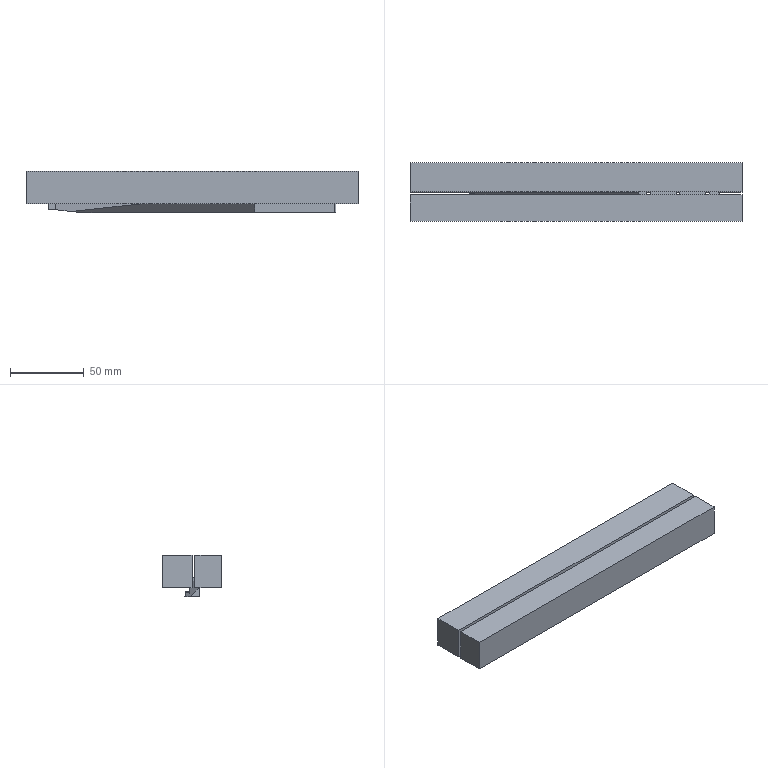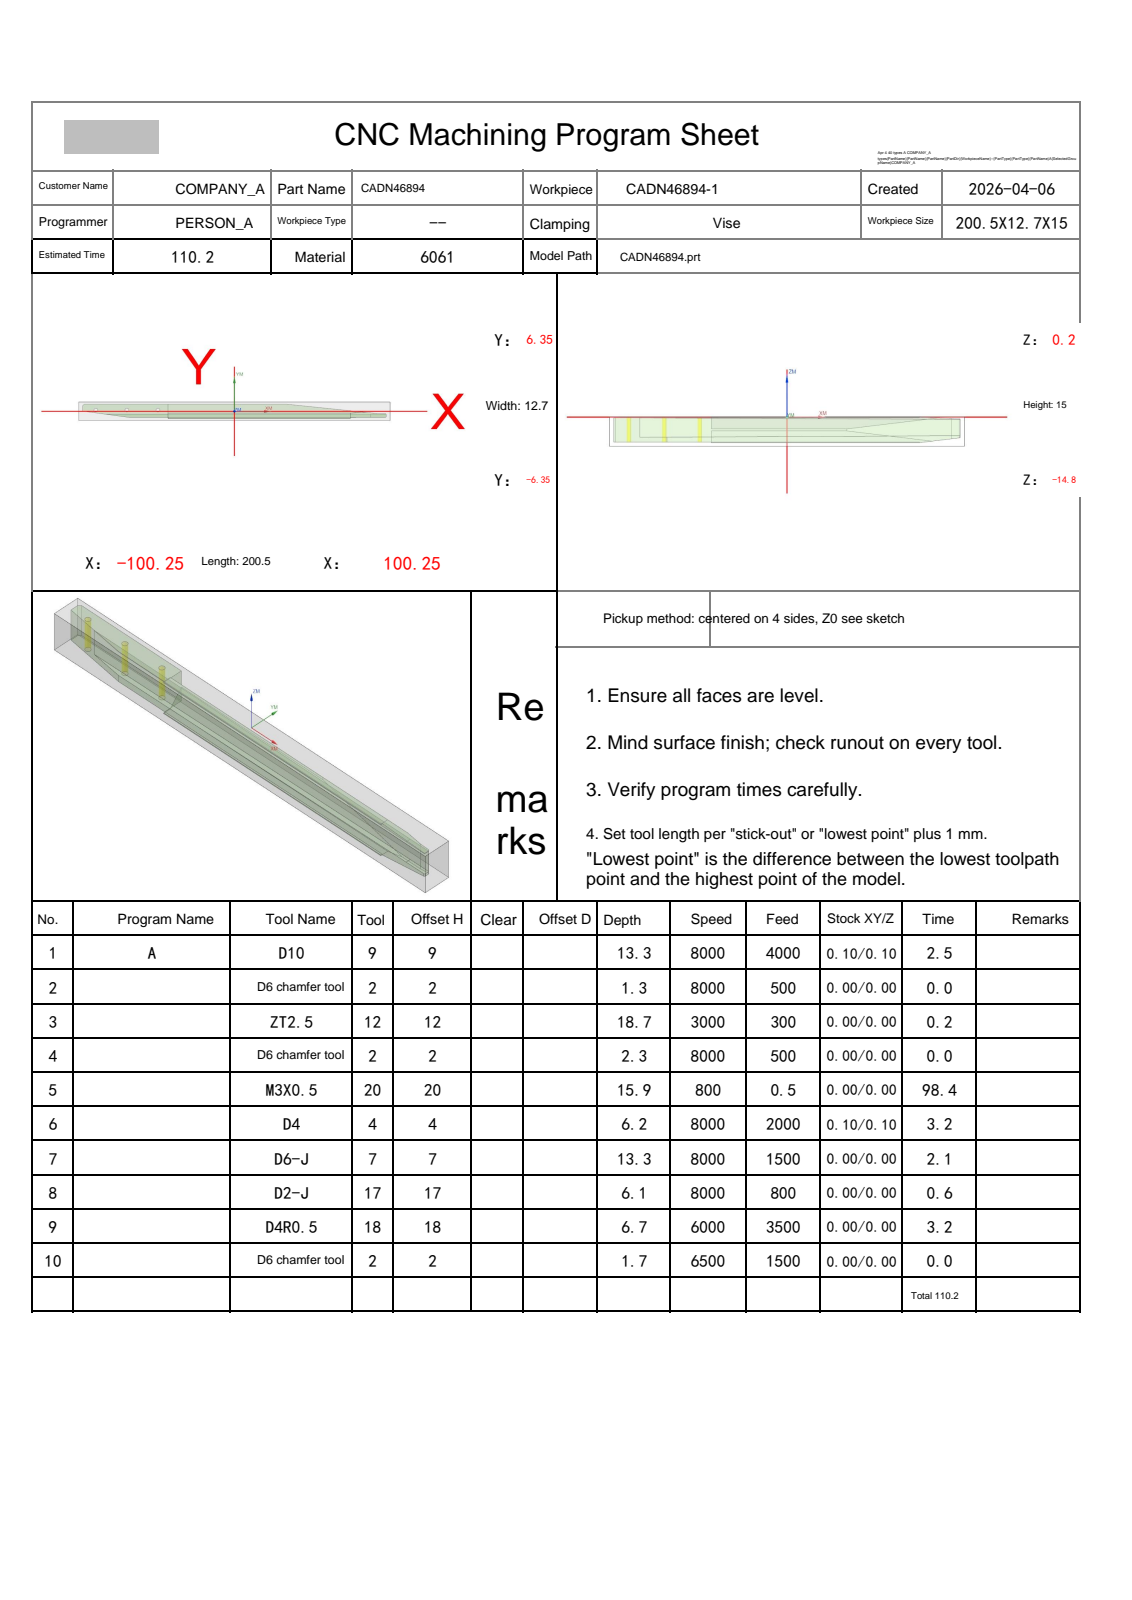NC program | NX | posted by the shop | part box 225.5 x 39.7 x 28 mm
Lines 1 to 2327 of 2996, first 1800 of 2325 lines:
%
O0001
(Machine time: 10.65 MIN)
(===Total Tool:5===)
(T4=D4      D=4.   R=0.   D-  H04 Z=-6.   )
(T7=D6-J    D=6.   R=0.   D7  H07 Z=-0.3  )
(T17=D2-J   D=2.   R=0.   D-  H17 Z=-5.9  )
(T2=D6 chamfer tool   D=6.   R=0.   D-  H02 Z=-1.5  )
(T18=D4R0.5 D=4.   R=0.5  D-  H18 Z=-6.43 )
G80 G90 G17 G49 G40
G91 G28 Z0
M01
N1 T04 M06
(D4  D=4. R=0. H=04 ce=0.20 di=0.10)
G00 G90 G54 X-209.5 Y-.74 M03 S4500
G43 H04 Z50.
M08
Z3.729
G01 Z1.729 F3000.
X-197.5
X1.601
G02 X2. Y-1.139 I-.001 J-.4
G01 Y-3.08
G02 X1.6 Y-3.48 I-.4 J0.0
G01 X-197.101
G03 X-197.5 Y-3.879 I.001 J-.4
G01 Y-5.86
G03 X-197.14 Y-6.22 I.36 J0.0
G01 X1.601
G02 X2. Y-6.619 I-.001 J-.4
G01 Y-8.56
G02 X1.6 Y-8.96 I-.4 J0.0
G01 X-197.5
X-209.5
Z3.729
G00 Z5.
Y-.74
Z3.457
G01 Z1.457
X-197.5
X1.601
G02 X2. Y-1.139 I-.001 J-.4
G01 Y-3.08
G02 X1.6 Y-3.48 I-.4 J0.0
G01 X-197.101
G03 X-197.5 Y-3.879 I.001 J-.4
G01 Y-5.86
G03 X-197.14 Y-6.22 I.36 J0.0
G01 X1.601
G02 X2. Y-6.619 I-.001 J-.4
G01 Y-8.56
G02 X1.6 Y-8.96 I-.4 J0.0
G01 X-197.5
X-209.5
Z3.457
G00 Z4.729
Y-.74
Z3.186
G01 Z1.186
X-197.5
X1.601
G02 X2. Y-1.139 I-.001 J-.4
G01 Y-3.08
G02 X1.6 Y-3.48 I-.4 J0.0
G01 X-197.101
G03 X-197.5 Y-3.879 I.001 J-.4
G01 Y-5.86
G03 X-197.14 Y-6.22 I.36 J0.0
G01 X1.601
G02 X2. Y-6.619 I-.001 J-.4
G01 Y-8.56
G02 X1.6 Y-8.96 I-.4 J0.0
G01 X-197.5
X-209.5
Z3.186
G00 Z4.457
Y-.74
Z2.914
G01 Z.914
X-197.5
X1.601
G02 X2. Y-1.139 I-.001 J-.4
G01 Y-3.08
G02 X1.6 Y-3.48 I-.4 J0.0
G01 X-197.101
G03 X-197.5 Y-3.879 I.001 J-.4
G01 Y-5.86
G03 X-197.14 Y-6.22 I.36 J0.0
G01 X1.601
G02 X2. Y-6.619 I-.001 J-.4
G01 Y-8.56
G02 X1.6 Y-8.96 I-.4 J0.0
G01 X-197.5
X-209.5
Z2.914
G00 Z4.186
Y-.74
Z2.643
G01 Z.643
X-197.5
X1.601
G02 X2. Y-1.139 I-.001 J-.4
G01 Y-3.08
G02 X1.6 Y-3.48 I-.4 J0.0
G01 X-197.101
G03 X-197.5 Y-3.879 I.001 J-.4
G01 Y-5.86
G03 X-197.14 Y-6.22 I.36 J0.0
G01 X1.601
G02 X2. Y-6.619 I-.001 J-.4
G01 Y-8.56
G02 X1.6 Y-8.96 I-.4 J0.0
G01 X-197.5
X-209.5
Z2.643
G00 Z3.914
Y-.74
Z2.371
G01 Z.371
X-197.5
X1.601
G02 X2. Y-1.139 I-.001 J-.4
G01 Y-3.08
G02 X1.6 Y-3.48 I-.4 J0.0
G01 X-197.101
G03 X-197.5 Y-3.879 I.001 J-.4
G01 Y-5.86
G03 X-197.14 Y-6.22 I.36 J0.0
G01 X1.601
G02 X2. Y-6.619 I-.001 J-.4
G01 Y-8.56
G02 X1.6 Y-8.96 I-.4 J0.0
G01 X-197.5
X-209.5
Z2.371
G00 Z3.643
Y-.74
Z2.1
G01 Z.1
X-197.5
X1.601
G02 X2. Y-1.139 I-.001 J-.4
G01 Y-3.08
G02 X1.6 Y-3.48 I-.4 J0.0
G01 X-197.101
G03 X-197.5 Y-3.879 I.001 J-.4
G01 Y-5.86
G03 X-197.14 Y-6.22 I.36 J0.0
G01 X1.601
G02 X2. Y-6.619 I-.001 J-.4
G01 Y-8.56
G02 X1.6 Y-8.96 I-.4 J0.0
G01 X-197.5
X-209.5
Z2.1
G00 Z50.
G00 G90 X-196.166 Y-14.577 M03 S8000
Z11.8
Z1.3
G01 Z-.2 F4000.
X-196.501 Y-10.471
G02 X-196.68 Y-6.08 I53.821 J4.391
G01 Y-3.536
G02 X-196.337 Y-3.14 I.4 J0.0
G01 X-194.045 Y-2.811
X-194. Y-2.808
G02 X-193.68 Y-3.128 I0.0 J-.32
G01 Y-6.08
G03 X-193.412 Y-11.301 I51. J0.0
X-193.014 Y-11.66 I.398 J.041
G01 X-190.713
G03 X-190.393 Y-11.34 I0.0 J.32
G01 X-190.395 Y-11.305
G02 X-190.68 Y-6.08 I47.715 J5.225
G01 Y-2.676
G02 X-190.337 Y-2.28 I.4 J0.0
G01 X-188.045 Y-1.951
X-188. Y-1.948
G02 X-187.68 Y-2.268 I0.0 J-.32
G01 Y-6.08
G03 X-187.375 Y-11.307 I45. J0.0
X-186.978 Y-11.66 I.397 J.047
G01 X-184.672
G03 X-184.352 Y-11.34 I0.0 J.32
G01 X-184.354 Y-11.3
G02 X-184.68 Y-6.08 I41.674 J5.22
G01 Y-1.816
G02 X-184.337 Y-1.42 I.4 J0.0
G01 X-182.045 Y-1.091
X-182. Y-1.088
G02 X-181.68 Y-1.408 I0.0 J-.32
G01 Y-6.08
G03 X-181.327 Y-11.314 I39. J0.0
X-180.931 Y-11.66 I.396 J.054
G01 X-178.617
G03 X-178.297 Y-11.34 I0.0 J.32
G01 X-178.3 Y-11.294
G02 X-178.68 Y-6.08 I35.62 J5.214
G01 Y-.956
G02 X-178.337 Y-.56 I.4 J0.0
G01 X-176.045 Y-.231
X-176. Y-.228
G02 X-175.68 Y-.548 I0.0 J-.32
G01 Y-6.08
G03 X-175.261 Y-11.324 I33. J0.0
X-174.866 Y-11.66 I.395 J.064
G01 X-172.54
G03 X-172.22 Y-11.34 I0.0 J.32
G01 X-172.225 Y-11.285
G02 X-172.68 Y-6.08 I29.545 J5.205
G01 Y-.096
G02 X-172.337 Y.3 I.4 J0.0
G01 X-170.045 Y.629
X-170. Y.632
G02 X-169.68 Y.312 I0.0 J-.32
G01 Y-6.08
G03 X-169.163 Y-11.338 I27. J0.0
X-168.771 Y-11.66 I.392 J.078
G01 X-166.374
G03 X-166.094 Y-11.38 I0.0 J.28
G01 X-166.101 Y-11.319
G02 X-166.68 Y-6.08 I23.421 J5.239
G01 Y.764
G02 X-166.337 Y1.16 I.4 J0.0
G01 X-165.668 Y1.256
X-165.611 Y1.26
X-164.08
G02 X-163.68 Y.86 I0.0 J-.4
G01 Y-6.08
G03 X-163.005 Y-11.361 I21. J0.0
X-162.618 Y-11.66 I.387 J.101
G01 X-160.175
G03 X-159.895 Y-11.38 I0.0 J.28
G01 X-159.907 Y-11.299
G02 X-160.68 Y-6.08 I17.227 J5.219
G01 Y.86
G02 X-160.28 Y1.26 I.4 J0.0
G01 X-158.08
G02 X-157.68 Y.86 I0.0 J-.4
G01 Y-6.08
G03 X-156.704 Y-11.402 I15. J0.0
X-156.33 Y-11.66 I.374 J.142
G01 X-153.694
G03 X-153.454 Y-11.42 I0.0 J.24
G01 X-153.478 Y-11.315
G02 X-154.68 Y-6.08 I10.798 J5.235
G01 Y.86
G02 X-154.28 Y1.26 I.4 J0.0
G01 X-152.08
G02 X-151.68 Y.86 I0.0 J-.4
G01 Y-6.08
G03 X-149.864 Y-11.501 I9. J0.0
X-149.545 Y-11.66 I.319 J.241
G01 X-145.272
X-145.192 Y-11.58
X-145.237 Y-11.508
G02 X-148.68 Y-6.08 I2.557 J5.428
G01 Y.86
G02 X-148.28 Y1.26 I.4 J0.0
G01 X-146.08
G02 X-145.68 Y.86 I0.0 J-.4
G01 Y-6.08
G03 X-142.68 Y-9.08 I3. J0.0
G01 X-138.882
G03 X-138.487 Y-8.742 I0.0 J.4
G01 X-138.145 Y-6.542
X-138.14 Y-6.48
G03 X-138.54 Y-6.08 I-.4 J0.0
G01 X-142.68
Y1.26
Y5.18
Z1.3
G00 Z11.8
G00 G90 X-88.285 Y-14.646 M03 S8000
Z11.8
Z.9
G01 Z-.3 F2000.
Y-14.2
G03 X-91.085 Y-11.4 I-2.8 J0.0
G01 X-138.458
G02 X-138.92 Y-11.836 I-2.056 J1.714
G01 X-140.071
X-140.147 Y-11.849
X-140.15 Y-11.771
G03 X-138.398 Y-9.686 I-.365 J2.085
G01 X-138.4 Y-9.589
X-138.321 Y-9.588
X-138.324 Y-6.236
X-138.333 Y-6.141
X-19.589
X-19.473 Y-6.145
G03 X-17.315 Y-4.099 I0.0 J2.162
G01 Y-.78
Y-.62
X.975
X1.83 Y-.628
X1.896 Y-.608
X1.903 Y-.677
X2.083 Y-1.121
X2.091 Y-1.226
Y-2.343
X2.08 Y-2.904
X2.066 Y-3.114
X2.084 Y-3.176
X2.019 Y-3.181
X1.867 Y-3.25
X1.561 Y-3.374
X1.531 Y-3.38
X-2.97 Y-3.379
X-12.736 Y-4.438
X-12.779 Y-4.44
G02 X-12.98 Y-4.386 I0.0 J.4
G01 X-14.792 Y-3.332
G03 X-14.993 Y-3.278 I-.201 J-.346
G01 X-15.105 Y-3.294
X-15.195 Y-3.307
G02 X-15.515 Y-2.988 I0.0 J.32
G01 Y-2.779
G02 X-15.156 Y-2.42 I.36 J-.002
G01 X-12.308
X-12.228 Y-2.5
X-12.299 Y-2.58
X-13.804 Y-2.743
G03 X-14.161 Y-3.141 I.043 J-.398
G01 X-14.159 Y-3.178
X-13.959 Y-5.302
X-13.957 Y-5.339
G02 X-14.064 Y-5.611 I-.4 J0.0
G01 X-14.205 Y-5.764
X-14.779 Y-6.274
X-15.027 Y-6.432
X-15.371 Y-6.524
X-15.942 Y-6.636
X-59.845 Y-11.4
X-93.085
G02 X-93.463 Y-11.129 I0.0 J.4
G01 X-93.892 Y-9.871
G03 X-94.27 Y-9.6 I-.378 J-.129
G01 X-136.123
G02 X-136.522 Y-9.202 I.002 J.4
G01 Y-8.34
G02 X-136.124 Y-7.941 I.4 J-.001
G01 X-46.135
X-46.056 Y-8.021
X-46.127 Y-8.101
X-59.962 Y-9.6
X-93.085
X-93.585
G03 X-96.385 Y-12.4 I0.0 J-2.8
G01 Y-14.645
Z.9
G00 Z3.
G01 X-89.675 Y-14.646 F6000.
G00 Z.6
G01 Z-.6 F2000.
Y-14.2
G03 X-92.475 Y-11.4 I-2.8 J0.0
G01 X-138.454
G02 X-138.915 Y-11.836 I-2.046 J1.7
G01 X-140.071
X-140.147 Y-11.849
X-140.15 Y-11.771
X-140.013 Y-11.743
G03 X-138.435 Y-10.083 I-.487 J2.043
X-138.398 Y-9.686 I-2.079 J.397
G01 X-138.4 Y-9.598
X-138.321 Y-9.597
X-138.322 Y-9.203
X-138.323 Y-7.001
X-138.324 Y-6.441
X-16.829
X-16.713 Y-6.445
G03 X-14.555 Y-4.399 I0.0 J2.162
G01 Y-.78
Y-.701
X-14.554 Y-.7
X-14.555 Y-.674
Y-.673
Y-.62
X.975
X1.83 Y-.628
X1.896 Y-.608
X1.903 Y-.677
X2.083 Y-1.121
X2.091 Y-1.226
Y-2.343
X2.08 Y-2.904
X2.066 Y-3.114
X2.084 Y-3.176
X2.019 Y-3.181
X1.867 Y-3.25
X1.561 Y-3.374
X1.531 Y-3.38
X-2.97 Y-3.379
X-11.332 Y-4.286
X-11.375 Y-4.288
G02 X-11.712 Y-4.104 I0.0 J.4
G01 X-12.577 Y-2.76
G03 X-12.722 Y-2.604 I-.499 J-.321
G01 X-12.781 Y-2.595
X-12.755 Y-2.541
Y-2.5
X-12.759 Y-2.415
X-12.675 Y-2.42
X-12.307
X-12.22 Y-2.419
X-12.189 Y-2.509
X-12.258 Y-2.563
X-12.35 Y-2.672
X-13.267 Y-4.325
G02 X-13.574 Y-4.528 I-.35 J.194
G01 X-13.761 Y-4.549
X-13.879 Y-5.147
X-13.96 Y-5.484
X-13.979 Y-5.52
X-14.205 Y-5.764
X-14.779 Y-6.274
X-15.027 Y-6.432
X-15.052 Y-6.439
X-15.371 Y-6.524
X-15.942 Y-6.636
X-19.31 Y-7.001
X-59.845 Y-11.4
X-94.475
G02 X-94.854 Y-11.129 I0.0 J.4
G01 X-95.283 Y-9.871
G03 X-95.661 Y-9.6 I-.378 J-.129
G01 X-136.124
G02 X-136.522 Y-9.202 I.002 J.4
G01 Y-8.64
G02 X-136.124 Y-8.241 I.4 J-.002
G01 X-48.9
X-48.821 Y-8.321
X-48.891 Y-8.401
X-59.962 Y-9.6
X-94.475
X-94.975
G03 X-97.775 Y-12.4 I0.0 J-2.8
G01 Y-14.644
Z.6
G00 Z2.7
G01 X-91.066 Y-14.646 F6000.
G00 Z.3
G01 Z-.9 F2000.
Y-14.2
G03 X-93.866 Y-11.4 I-2.8 J0.0
G01 X-138.454
G02 X-138.915 Y-11.836 I-2.046 J1.7
G01 X-140.071
X-140.147 Y-11.849
X-140.15 Y-11.771
X-140.013 Y-11.743
G03 X-138.435 Y-10.083 I-.487 J2.043
X-138.398 Y-9.686 I-2.079 J.397
G01 X-138.399 Y-9.607
X-138.321 Y-9.606
X-138.322 Y-9.204
X-138.323 Y-6.741
X-17.636
X-16.758 Y-6.688
X-15.524 Y-6.554
X-15.942 Y-6.636
X-59.845 Y-11.4
X-95.866
G02 X-96.244 Y-11.129 I0.0 J.4
G01 X-96.673 Y-9.871
G03 X-97.051 Y-9.6 I-.378 J-.129
G01 X-136.124
G02 X-136.522 Y-9.202 I.002 J.4
G01 Y-8.94
G02 X-136.124 Y-8.541 I.4 J-.002
G01 X-51.665
X-51.585 Y-8.621
X-51.656 Y-8.701
X-59.962 Y-9.6
X-95.866
X-96.366
G03 X-99.166 Y-12.4 I0.0 J-2.8
G01 Y-14.644
Z.3
G00 Z2.4
G01 X-92.476 Y-14.645 F6000.
G00 Z0.0
G01 Z-1.2 F2000.
Y-14.2
G03 X-95.276 Y-11.4 I-2.8 J0.0
G01 X-138.454
G02 X-138.915 Y-11.836 I-2.046 J1.7
G01 X-140.071
X-140.147 Y-11.849
X-140.15 Y-11.771
X-140.013 Y-11.743
G03 X-138.435 Y-10.083 I-.487 J2.043
X-138.398 Y-9.686 I-2.079 J.397
G01 X-138.399 Y-9.617
X-138.321 Y-9.616
X-138.322 Y-9.244
X-138.323 Y-7.041
X-20.402
X-19.336 Y-6.967
X-15.524 Y-6.554
X-15.533 Y-6.556
X-15.942 Y-6.636
X-24.839 Y-7.601
X-59.845 Y-11.4
X-97.276
G02 X-97.654 Y-11.129 I0.0 J.4
G01 X-98.084 Y-9.871
G03 X-98.462 Y-9.6 I-.378 J-.129
G01 X-136.164
G02 X-136.524 Y-9.238 I.002 J.362
G01 X-136.522 Y-9.2
G02 X-136.164 Y-8.841 I.36 J-.002
G01 X-54.429
X-54.35 Y-8.921
X-54.42 Y-9.001
X-59.959 Y-9.6
X-97.276
X-97.776
G03 X-100.576 Y-12.4 I0.0 J-2.8
G01 Y-14.644
Z0.0
G00 Z2.1
G01 X-93.946 Y-14.645 F6000.
G00 Z-.3
G01 Z-1.5 F2000.
Y-14.2
G03 X-96.746 Y-11.4 I-2.8 J0.0
G01 X-138.454
G02 X-138.915 Y-11.836 I-2.046 J1.7
G01 X-140.071
X-140.147 Y-11.849
X-140.15 Y-11.771
X-140.013 Y-11.743
G03 X-138.435 Y-10.083 I-.487 J2.043
X-138.398 Y-9.686 I-2.079 J.397
G01 X-138.399 Y-9.626
X-138.321 Y-9.625
X-138.322 Y-9.403
X-138.323 Y-7.341
X-23.167
X-21.593 Y-7.212
X-16.606 Y-6.671
X-15.524 Y-6.554
X-15.533 Y-6.556
X-15.942 Y-6.636
X-59.845 Y-11.4
X-98.746
G02 X-99.125 Y-11.129 I0.0 J.4
G01 X-99.554 Y-9.871
G03 X-99.932 Y-9.6 I-.378 J-.129
G01 X-136.323
G02 X-136.522 Y-9.402 I.002 J.2
G01 Y-9.34
G02 X-136.323 Y-9.141 I.2 J-.001
G01 X-57.194
X-57.115 Y-9.221
X-57.185 Y-9.301
X-59.951 Y-9.6
X-98.746
X-99.246
G03 X-102.046 Y-12.4 I0.0 J-2.8
G01 Y-14.644
Z-.3
G00 Z1.8
G01 X-74.061 Y-14.649 F6000.
G00 Z-.6
G01 Z-1.8 F2000.
Y-14.2
G03 X-76.861 Y-11.4 I-2.8 J0.0
G01 X-138.454
G02 X-138.915 Y-11.836 I-2.046 J1.7
G01 X-140.071
X-140.147 Y-11.849
X-140.15 Y-11.771
X-140.013 Y-11.743
G03 X-138.435 Y-10.083 I-.487 J2.043
X-138.398 Y-9.686 I-2.079 J.397
G01 Y-9.636
X-138.321 Y-9.634
X-138.323 Y-7.641
X-25.933
X-25.055 Y-7.588
X-16.015 Y-6.607
X-15.524 Y-6.554
X-15.533 Y-6.556
X-15.781 Y-6.604
X-15.942 Y-6.636
X-28.475 Y-7.996
X-30.369 Y-8.201
X-59.845 Y-11.4
X-76.861
X-77.361
G03 X-80.161 Y-14.2 I0.0 J-2.8
G01 Y-14.648
Z-.6
G00 Z1.5
G01 X-74.061 Y-14.649 F6000.
G00 Z-.9
G01 Z-2.1 F2000.
Y-14.2
G03 X-76.861 Y-11.4 I-2.8 J0.0
G01 X-138.454
G02 X-138.915 Y-11.836 I-2.046 J1.7
G01 X-140.071
X-140.147 Y-11.849
X-140.15 Y-11.771
X-140.013 Y-11.743
G03 X-138.435 Y-10.083 I-.487 J2.043
X-138.398 Y-9.686 I-2.079 J.397
G01 Y-9.645
X-138.321 Y-9.644
X-138.322 Y-8.81
Y-8.501
X-138.323 Y-7.941
X-28.699
X-27.821 Y-7.888
X-25.055 Y-7.588
X-22.1 Y-7.267
X-18.812 Y-6.911
X-15.524 Y-6.554
X-15.533 Y-6.556
X-15.942 Y-6.636
X-59.845 Y-11.4
X-76.861
X-77.361
G03 X-80.161 Y-14.2 I0.0 J-2.8
G01 Y-14.648
Z-.9
G00 Z1.2
G01 X-74.061 Y-14.649 F6000.
G00 Z-1.2
G01 Z-2.4 F2000.
Y-14.2
G03 X-76.861 Y-11.4 I-2.8 J0.0
G01 X-138.454
G02 X-138.915 Y-11.836 I-2.046 J1.7
G01 X-140.071
X-140.147 Y-11.849
X-140.15 Y-11.771
X-140.013 Y-11.743
G03 X-138.435 Y-10.083 I-.487 J2.043
X-138.398 Y-9.686 I-2.079 J.397
G01 Y-9.654
X-138.321 Y-9.653
X-138.322 Y-8.241
X-31.519
X-30.586 Y-8.188
X-16.998 Y-6.714
X-15.524 Y-6.554
X-15.533 Y-6.556
X-15.942 Y-6.636
X-59.845 Y-11.4
X-76.861
X-77.361
G03 X-80.161 Y-14.2 I0.0 J-2.8
G01 Y-14.648
Z-1.2
G00 Z.9
G01 X-84.266 Y-14.647 F6000.
G00 Z-1.5
G01 Z-2.7 F2000.
G03 X-87.066 Y-11.846 I-2.8 J0.0
G01 X-140.071 Y-11.836
X-140.147 Y-11.849
X-140.15 Y-11.771
X-140.013 Y-11.743
G03 X-138.435 Y-10.083 I-.487 J2.043
X-138.398 Y-9.686 I-2.079 J.397
G01 Y-9.664
X-138.32 Y-9.663
X-138.322 Y-8.541
X-34.244 Y-8.538
X-34.235 Y-8.621
X-63.905 Y-11.84
X-64.471 Y-11.851
X-87.066 Y-11.846
X-87.566
G03 X-90.366 Y-14.646 I0.0 J-2.8
G01 Z-1.5
G00 Z.6
G01 X-84.266 Y-14.647 F6000.
G00 Z-1.8
G01 Z-3. F2000.
G03 X-87.066 Y-11.846 I-2.8 J0.0
G01 X-140.071 Y-11.836
X-140.147 Y-11.849
X-140.15 Y-11.771
X-139.973 Y-11.733
G03 X-138.435 Y-10.083 I-.527 J2.033
X-138.398 Y-9.686 I-2.079 J.397
G01 Y-9.673
X-138.32 Y-9.672
X-138.321 Y-9.588
X-138.322 Y-8.841
X-37.144
X-37.008 Y-8.834
X-36.999 Y-8.921
X-63.905 Y-11.84
X-64.471 Y-11.851
X-87.066 Y-11.846
X-87.566
G03 X-90.366 Y-14.646 I0.0 J-2.8
G01 Z-1.8
G00 Z.3
G01 X-84.266 Y-14.647 F6000.
G00 Z-2.1
G01 Z-3.3 F2000.
G03 X-87.066 Y-11.846 I-2.8 J0.0
G01 X-140.071 Y-11.836
X-140.147 Y-11.849
X-140.15 Y-11.771
X-140.013 Y-11.743
G03 X-138.435 Y-10.083 I-.487 J2.043
X-138.398 Y-9.686 I-2.079 J.396
G01 Y-9.682
X-138.32 Y-9.681
X-138.321 Y-9.588
X-138.322 Y-9.141
X-39.919
X-39.773 Y-9.134
X-39.763 Y-9.221
X-63.905 Y-11.84
X-64.471 Y-11.851
X-87.066 Y-11.846
X-87.566
G03 X-90.366 Y-14.646 I0.0 J-2.8
G01 Z-2.1
G00 Z0.0
G01 X-84.266 Y-14.647 F6000.
G00 Z-2.4
G01 Z-3.6 F2000.
G03 X-87.066 Y-11.846 I-2.8 J0.0
G01 X-140.071 Y-11.836
X-140.147 Y-11.849
X-140.15 Y-11.771
X-140.013 Y-11.743
G03 X-138.435 Y-10.083 I-.487 J2.043
X-138.398 Y-9.692 I-2.079 J.396
G01 X-138.32 Y-9.691
X-138.321 Y-9.588
X-138.322 Y-9.441
X-42.537
X-42.528 Y-9.521
X-63.905 Y-11.84
X-64.471 Y-11.851
X-87.066 Y-11.846
X-87.566
G03 X-90.366 Y-14.646 I0.0 J-2.8
G01 Z-2.4
G00 Z-.3
G01 X-84.266 Y-14.647 F6000.
G00 Z-2.7
G01 Z-3.9 F2000.
G03 X-87.066 Y-11.846 I-2.8 J0.0
G01 X-140.071 Y-11.836
X-140.147 Y-11.849
X-140.15 Y-11.771
X-140.013 Y-11.743
G03 X-138.435 Y-10.083 I-.487 J2.043
X-138.398 Y-9.742 I-2.079 J.396
G01 X-138.325 Y-9.75
X-138.324 Y-9.741
X-45.302
X-45.293 Y-9.821
X-63.905 Y-11.84
X-64.471 Y-11.851
X-87.066 Y-11.846
X-87.566
G03 X-90.366 Y-14.646 I0.0 J-2.8
G01 Z-2.7
G00 Z-.6
G01 X-84.266 Y-14.647 F6000.
G00 Z-3.
G01 Z-4.2 F2000.
G03 X-87.066 Y-11.846 I-2.8 J0.0
G01 X-140.071 Y-11.836
X-140.147 Y-11.849
X-140.15 Y-11.771
G03 X-139.954 Y-11.728 I-.362 J2.086
X-138.428 Y-10.043 I-.546 J2.028
G01 X-138.357 Y-10.05
X-138.356 Y-10.041
X-48.066
X-48.058 Y-10.121
X-63.905 Y-11.84
X-64.471 Y-11.851
X-87.066 Y-11.846
X-87.566
G03 X-90.366 Y-14.646 I0.0 J-2.8
G01 Z-3.
G00 Z-.9
G01 X-84.266 Y-14.647 F6000.
G00 Z-3.3
G01 Z-4.5 F2000.
G03 X-87.066 Y-11.846 I-2.8 J0.0
G01 X-140.071 Y-11.836
X-140.147 Y-11.849
X-140.15 Y-11.771
X-140.013 Y-11.743
G03 X-138.5 Y-10.342 I-.487 J2.043
G01 X-138.425 Y-10.363
X-138.419 Y-10.341
X-50.831
X-50.822 Y-10.421
X-63.905 Y-11.84
X-64.471 Y-11.851
X-87.066 Y-11.846
X-87.566
G03 X-90.366 Y-14.646 I0.0 J-2.8
G01 Z-3.3
G00 Z-1.2
G01 X-84.266 Y-14.647 F6000.
G00 Z-3.6
G01 Z-4.8 F2000.
G03 X-87.066 Y-11.846 I-2.8 J0.0
G01 X-140.071 Y-11.836
X-140.147 Y-11.849
X-140.15 Y-11.771
X-140.013 Y-11.743
G03 X-138.624 Y-10.644 I-.487 J2.043
G01 X-138.555 Y-10.674
X-138.541 Y-10.641
X-53.596
X-53.587 Y-10.721
X-63.905 Y-11.84
X-64.471 Y-11.851
X-87.066 Y-11.846
X-87.566
G03 X-90.366 Y-14.646 I0.0 J-2.8
G01 Z-3.6
G00 Z-1.5
G01 X-84.266 Y-14.647 F6000.
G00 Z-3.9
G01 Z-5.1 F2000.
G03 X-87.066 Y-11.846 I-2.8 J0.0
G01 X-140.071 Y-11.836
X-140.147 Y-11.849
X-140.15 Y-11.771
X-140.013 Y-11.743
G03 X-138.808 Y-10.943 I-.487 J2.043
G01 X-138.744 Y-10.992
X-138.711 Y-10.941
X-56.36
X-56.351 Y-11.021
X-63.905 Y-11.84
X-64.471 Y-11.851
X-87.066 Y-11.846
X-87.566
G03 X-90.366 Y-14.646 I0.0 J-2.8
G01 Z-3.9
G00 Z-1.8
G01 X-84.266 Y-14.647 F6000.
G00 Z-4.2
G01 Z-5.4 F2000.
G03 X-87.066 Y-11.846 I-2.8 J0.0
G01 X-140.071 Y-11.836
X-140.147 Y-11.849
X-140.15 Y-11.771
X-140.013 Y-11.743
G03 X-139.074 Y-11.242 I-.487 J2.043
G01 X-139.018 Y-11.298
X-138.962 Y-11.241
X-59.125 Y-11.239
X-59.116 Y-11.321
X-63.905 Y-11.84
X-64.471 Y-11.851
X-87.066 Y-11.846
X-87.566
G03 X-90.366 Y-14.646 I0.0 J-2.8
G01 Z-4.2
G00 Z-2.1
G01 X-84.266 Y-14.647 F6000.
G00 Z-4.5
G01 Z-5.7 F2000.
G03 X-87.066 Y-11.846 I-2.8 J0.0
G01 X-140.071 Y-11.836
X-140.147 Y-11.849
X-140.15 Y-11.771
X-140.013 Y-11.743
G03 X-139.485 Y-11.541 I-.478 J2.048
G01 X-139.454 Y-11.615
X-139.277 Y-11.541
X-61.89 Y-11.538
X-61.881 Y-11.621
X-63.905 Y-11.84
X-64.471 Y-11.851
X-87.066 Y-11.846
X-87.566
G03 X-90.366 Y-14.646 I0.0 J-2.8
G01 Z-4.5
G00 Z-2.4
G01 X-84.266 Y-14.647 F6000.
G00 Z-4.8
G01 Z-6. F2000.
G03 X-87.066 Y-11.846 I-2.8 J0.0
G01 X-140.071 Y-11.836
X-140.128 Y-11.862
X-140.138 Y-11.8
X-63.886
X-61.885 Y-11.583
X-61.881 Y-11.621
X-63.905 Y-11.84
X-64.471 Y-11.851
X-87.066 Y-11.846
X-87.566
G03 X-90.366 Y-14.646 I0.0 J-2.8
G01 Z-4.8
G00 Z11.8
X-7.782 Y6.3
Z.3
G01 Z-.9
Y2.18
G03 X-4.982 Y-.62 I2.8 J0.0
G01 X.975
X1.83 Y-.628
X1.896 Y-.608
X1.903 Y-.677
X2.083 Y-1.121
X2.091 Y-1.226
Y-2.343
X2.08 Y-2.904
X2.066 Y-3.114
X2.084 Y-3.176
X2.019 Y-3.181
X1.867 Y-3.25
X1.561 Y-3.374
X1.531 Y-3.38
X-2.97 Y-3.379
X-11.798 Y-4.336
X-11.795 Y-4.255
Y-.78
Y-.62
X-4.982
X-4.482
G03 X-1.682 Y2.18 I0.0 J2.8
G01 Y6.3
Z.3
G00 Z2.4
G01 X-7.782 F6000.
G00 Z0.0
G01 Z-1.2 F2000.
Y2.18
G03 X-4.982 Y-.62 I2.8 J0.0
G01 X.975
X1.83 Y-.628
X1.896 Y-.608
X1.903 Y-.677
X2.083 Y-1.121
X2.091 Y-1.226
Y-2.343
X2.08 Y-2.904
X2.066 Y-3.114
X2.084 Y-3.176
X2.019 Y-3.181
X1.867 Y-3.25
X1.561 Y-3.374
X1.531 Y-3.38
X-2.97 Y-3.379
X-9.038 Y-4.037
X-9.035 Y-3.956
Y-.78
Y-.62
X-4.982
X-4.482
G03 X-1.682 Y2.18 I0.0 J2.8
G01 Y6.3
Z0.0
G00 Z2.1
G01 X-6.382 F6000.
G00 Z-.3
G01 Z-1.5 F2000.
Y.78
G03 X-4.982 Y-.62 I1.4 J0.0
G01 X.975
X1.83 Y-.628
X1.896 Y-.608
X1.903 Y-.677
X2.083 Y-1.121
X2.091 Y-1.226
Y-2.343
X2.08 Y-2.904
X2.066 Y-3.114
X2.084 Y-3.176
X2.019 Y-3.181
X1.867 Y-3.25
X1.561 Y-3.374
X1.531 Y-3.38
X-2.97 Y-3.379
X-6.278 Y-3.738
X-6.275 Y-3.656
Y-.78
Y-.7
Y-.641
Y-.62
X-4.982
X-4.482
G03 X-1.682 Y2.18 I0.0 J2.8
G01 Y6.3
Z-.3
G00 Z1.8
G01 X-3.642 F6000.
G00 Z-.6
G01 Z-1.8 F2000.
Y2.18
G03 X-.842 Y-.62 I2.8 J0.0
G01 X.975
X1.83 Y-.628
X1.896 Y-.608
X1.903 Y-.677
X2.083 Y-1.121
X2.091 Y-1.226
Y-2.343
X2.08 Y-2.904
X2.066 Y-3.114
X2.084 Y-3.176
X2.019 Y-3.181
X1.867 Y-3.25
X1.561 Y-3.374
X1.531 Y-3.38
X-2.97 Y-3.379
X-3.566 Y-3.444
X-3.515 Y-3.357
Y-.78
Y-.7
Y-.646
Y-.62
X-.842
X-.342
G03 X2.458 Y2.18 I0.0 J2.8
G01 Y6.3
Z-.6
G00 Z3.
G01 X1.049 Y-2.476 F6000.
G00 Z-.3
G02 X1.049 Y-2.476 Z-.893 I.996 J1.499 F2000.
X1.049 Y-2.476 Z-1.485 I.996 J1.499
X1.049 Y-2.476 Z-2.078 I.996 J1.499
X.732 Y-2.207 Z-2.1 I.996 J1.499
G01 X-.755 Y-.62
X.975
X1.83 Y-.628
X1.896 Y-.608
X1.903 Y-.677
X2.083 Y-1.121
X2.091 Y-1.226
Y-2.343
X2.08 Y-2.904
X2.066 Y-3.114
X2.084 Y-3.176
X2.019 Y-3.181
X1.867 Y-3.25
X1.561 Y-3.374
X1.531 Y-3.38
X-.756
X-.755 Y-3.3
Y-.78
Y-.62
X-.255
G03 X2.545 Y2.18 I0.0 J2.8
G01 Y6.3
Z-.9
G00 Z1.2
G01 X7.015 Y.669 F6000.
G00 Z-1.2
G01 Z-2.4 F2000.
X4.891
G03 X2.091 Y-2.131 I0.0 J-2.8
G01 Y-2.343
X2.08 Y-2.904
X2.066 Y-3.114
X2.084 Y-3.176
X2.019 Y-3.181
X1.979 Y-3.199
G03 X2.005 Y-2.873 I-2.545 J.371
G01 Y-1.155
X2.085 Y-1.149
X2.091 Y-1.226
Y-2.131
Y-2.341
X2.085 Y-2.631
Y-2.684
G03 X4.833 Y-5.483 I2.8 J0.0
G01 X7.3 Y-5.529
Z-1.2
G00 Z11.8
G91 G28 Z0.0
M05
M09
G91 G28 Z0.0
M01
N2 T07 M06
(D6-J  D=6. R=0. H=07 ce=0.00 di=0.00)
G00 G90 G54 X-210.5 Y-.925 M03 S8000
G43 H07 Z50.
M08
Z2.
G01 Z0.0 F1000.
X-198.5
X3.
Y-4.85
X-198.5
Y-8.775
X3.
X15.
Z2.
G00 Z50.
G00 G90 X-169.024 Y-13.9 M03 S7000
Z11.8
Z1.2
G01 Z-.3 F1500.
Y-11.5
G03 X-170.224 Y-10.3 I-1.2 J0.0
G01 X-194.502
G02 X-194.923 Y-10.125 I.002 J.6
G01 X-195.925 Y-9.123
G02 X-196.1 Y-8.7 I.425 J.423
G01 Y-4.998
G02 X-195.587 Y-4.406 I.6 J-.002
G01 X-165.584 Y-.106
X-165.502 Y-.1
X-144.498
G02 X-143.9 Y-.698 I-.002 J-.6
G01 Y-9.702
G02 X-144.498 Y-10.3 I-.6 J.002
G01 X-171.475
G02 X-171.899 Y-10.124 I0.0 J.6
G01 X-174.548 Y-7.476
G03 X-174.972 Y-7.3 I-.424 J-.424
G01 X-192.949
X-193.068 Y-7.18
X-192.966 Y-7.061
X-165.37 Y-3.106
X-165.288 Y-3.1
X-147.498
G02 X-146.9 Y-3.698 I-.002 J-.6
G01 Y-6.702
G02 X-147.498 Y-7.3 I-.6 J.002
G01 X-173.224
X-174.224
G03 X-175.424 Y-8.5 I0.0 J-1.2
G01 Y-13.9
Z1.2
G00 Z11.8
G00 G90 X-144.9 Y-13.9 M03 S8000
Z11.8
Z.7
G01 Z-.3 F1000.
G41 D07
X-144.7
G03 X-143.5 Y-12.7 I0.0 J1.2
G01 Y2.3
G03 X-144.7 Y3.5 I-1.2 J0.0
G01 G40 X-144.9
Z.7
G00 Z11.8
G91 G28 Z0.0
M05
M09
G91 G28 Z0.0
M01
N3 T17 M06
(D2-J  D=2. R=0. H=17 ce=0.00 di=0.00)
G00 G90 G54 X-135.35 Y-5.242 M03 S8000
G43 H17 Z50.
M08
Z-.058
G01 X-135.351 Y-5.24 Z-.093 F800.
X-135.353 Y-5.234 Z-.128
X-135.357 Y-5.225 Z-.162
X-135.362 Y-5.214 Z-.196
X-135.369 Y-5.2 Z-.229
X-135.379 Y-5.186 Z-.26
X-135.39 Y-5.171 Z-.289
X-135.405 Y-5.156 Z-.316
X-135.421 Y-5.141 Z-.34
X-135.441 Y-5.128 Z-.36
X-135.463 Y-5.117 Z-.377
X-135.489 Y-5.108 Z-.389
X-135.518 Y-5.102 Z-.397
X-135.551 Y-5.1 Z-.4
X-139.5
Y-9.05
X-139.486 Y-9.064
X-139.444 Y-9.053
X-139.379 Y-9.02 Z-.399
X-139.291 Y-8.966 Z-.398
X-138.935 Y-8.704 Z-.395
X-138.623 Y-8.453 Z-.392
X-138.39 Y-8.256 Z-.39
X-138.126 Y-8.023 Z-.388
X-137.827 Y-7.749 Z-.386
X-137.506 Y-7.445
X-137.18 Y-7.124 Z-.388
X-136.871 Y-6.81 Z-.393
X-136.593 Y-6.518 Z-.401
X-136.356 Y-6.262 Z-.412
X-136.156 Y-6.037 Z-.425
X-135.901 Y-5.737 Z-.448
X-135.636 Y-5.397 Z-.479
X-135.581 Y-5.314 Z-.487
X-135.547 Y-5.252 Z-.494
X-135.536 Y-5.213 Z-.498
X-135.55 Y-5.2 Z-.5
X-139.5
Y-9.15
X-139.486 Y-9.164
X-139.444 Y-9.153
X-139.379 Y-9.12 Z-.499
X-139.291 Y-9.066 Z-.498
X-138.935 Y-8.804 Z-.495
X-138.623 Y-8.553 Z-.492
X-138.39 Y-8.356 Z-.49
X-138.126 Y-8.123 Z-.488
X-137.827 Y-7.849 Z-.486
X-137.506 Y-7.545
X-137.18 Y-7.224 Z-.488
X-136.871 Y-6.91 Z-.493
X-136.593 Y-6.618 Z-.501
X-136.356 Y-6.362 Z-.512
X-136.156 Y-6.137 Z-.525
X-135.901 Y-5.837 Z-.548
X-135.636 Y-5.497 Z-.579
X-135.581 Y-5.414 Z-.587
X-135.547 Y-5.352 Z-.594
X-135.536 Y-5.313 Z-.598
X-135.551 Y-5.3 Z-.6
X-139.5
Y-9.25
X-139.486 Y-9.264
X-139.445 Y-9.253
X-139.379 Y-9.22 Z-.599
X-139.292 Y-9.166 Z-.598
X-138.936 Y-8.904 Z-.595
X-138.624 Y-8.653 Z-.592
X-138.392 Y-8.456 Z-.59
X-138.128 Y-8.223 Z-.588
X-137.831 Y-7.949 Z-.586
X-137.511 Y-7.645
X-137.185 Y-7.324 Z-.588
X-136.876 Y-7.01 Z-.593
X-136.599 Y-6.718 Z-.601
X-136.363 Y-6.462 Z-.612
X-136.163 Y-6.237 Z-.625
X-135.909 Y-5.937 Z-.648
X-135.645 Y-5.597 Z-.679
X-135.59 Y-5.514 Z-.687
X-135.556 Y-5.452 Z-.694
X-135.545 Y-5.413 Z-.698
X-135.56 Y-5.4 Z-.7
X-139.5
Y-9.268
X-139.486 Y-9.282
X-139.445 Y-9.273
X-139.379 Y-9.24 Z-.699
X-139.292 Y-9.188 Z-.698
X-138.935 Y-8.933 Z-.695
X-138.623 Y-8.688 Z-.692
X-138.391 Y-8.495 Z-.69
X-138.127 Y-8.267 Z-.687
X-137.829 Y-7.999 Z-.686
X-137.508 Y-7.701
X-137.183 Y-7.387 Z-.688
X-136.873 Y-7.079 Z-.693
X-136.596 Y-6.794 Z-.701
X-136.359 Y-6.542 Z-.712
X-136.159 Y-6.321 Z-.725
X-135.905 Y-6.027 Z-.748
X-135.64 Y-5.694 Z-.779
X-135.585 Y-5.612 Z-.787
X-135.551 Y-5.551 Z-.794
X-135.54 Y-5.513 Z-.798
X-135.555 Y-5.5 Z-.8
X-139.5
Y-9.411
X-139.486 Y-9.426
X-139.445 Y-9.416
X-139.379 Y-9.383 Z-.799
X-139.292 Y-9.329 Z-.798
X-138.935 Y-9.071 Z-.795
X-138.623 Y-8.823 Z-.792
X-138.39 Y-8.627 Z-.79
X-138.126 Y-8.397 Z-.788
X-137.828 Y-8.126 Z-.786
X-137.507 Y-7.824
X-137.181 Y-7.507 Z-.788
X-136.871 Y-7.195 Z-.793
X-136.594 Y-6.907 Z-.802
X-136.357 Y-6.652 Z-.812
X-136.157 Y-6.43 Z-.825
X-135.902 Y-6.133 Z-.848
X-135.637 Y-5.795 Z-.879
X-135.582 Y-5.713 Z-.887
X-135.548 Y-5.652 Z-.894
X-135.537 Y-5.613 Z-.898
X-135.552 Y-5.6 Z-.9
X-139.5
Y-9.54
X-139.486 Y-9.554
X-139.444 Y-9.543
X-139.379 Y-9.51 Z-.899
X-139.291 Y-9.456 Z-.898
X-138.935 Y-9.196 Z-.895
X-138.623 Y-8.945 Z-.892
X-138.39 Y-8.749 Z-.89
X-138.126 Y-8.516 Z-.888
X-137.827 Y-8.243 Z-.886
X-137.506 Y-7.939
X-137.18 Y-7.62 Z-.888
X-136.871 Y-7.306 Z-.893
X-136.593 Y-7.015 Z-.902
X-136.356 Y-6.759 Z-.912
X-136.156 Y-6.535 Z-.925
X-135.901 Y-6.236 Z-.948
X-135.636 Y-5.897 Z-.979
X-135.581 Y-5.814 Z-.987
X-135.547 Y-5.752 Z-.994
X-135.536 Y-5.713 Z-.998
X-135.551 Y-5.7 Z-1.
X-139.5
Y-9.65
X-139.486 Y-9.664
X-139.445 Y-9.653
X-139.379 Y-9.62 Z-.999
X-139.292 Y-9.566 Z-.998
X-138.935 Y-9.304 Z-.995
X-138.623 Y-9.053 Z-.992
X-138.39 Y-8.856 Z-.99
X-138.126 Y-8.623 Z-.988
X-137.828 Y-8.349 Z-.986
X-137.507 Y-8.044
X-137.181 Y-7.724 Z-.988
X-136.871 Y-7.41 Z-.993
X-136.593 Y-7.118 Z-1.002
X-136.357 Y-6.862 Z-1.012
X-136.157 Y-6.637 Z-1.025
X-135.902 Y-6.337 Z-1.048
X-135.637 Y-5.997 Z-1.079
X-135.582 Y-5.914 Z-1.087
X-135.548 Y-5.852 Z-1.094
X-135.537 Y-5.813 Z-1.098
X-135.552 Y-5.8 Z-1.1
X-139.5
Y-9.7
X-139.486 Y-9.714
X-139.445 Y-9.704
X-139.379 Y-9.672 Z-1.099
X-139.292 Y-9.618 Z-1.098
X-138.935 Y-9.361 Z-1.095
X-138.623 Y-9.114 Z-1.092
X-138.391 Y-8.919 Z-1.09
X-138.127 Y-8.689 Z-1.088
X-137.829 Y-8.419 Z-1.086
X-137.508 Y-8.118
X-137.183 Y-7.802 Z-1.088
X-136.873 Y-7.491 Z-1.093
X-136.596 Y-7.203 Z-1.102
X-136.359 Y-6.95 Z-1.112
X-136.159 Y-6.727 Z-1.125
X-135.905 Y-6.431 Z-1.148
X-135.64 Y-6.095 Z-1.179
X-135.585 Y-6.013 Z-1.187
X-135.551 Y-5.952 Z-1.194
X-135.54 Y-5.913 Z-1.198
X-135.555 Y-5.9 Z-1.2
X-139.5
Y-9.7
X-139.486 Y-9.715
X-139.445 Y-9.705
X-139.379 Y-9.674 Z-1.199
X-139.292 Y-9.623 Z-1.198
X-138.998 Y-9.42 Z-1.195
X-138.638 Y-9.144 Z-1.192
X-138.392 Y-8.944 Z-1.19
X-138.129 Y-8.72 Z-1.188
X-137.831 Y-8.457 Z-1.186
X-137.511 Y-8.164
X-137.186 Y-7.856 Z-1.188
X-136.876 Y-7.553 Z-1.193
X-136.599 Y-7.272 Z-1.202
X-136.363 Y-7.025 Z-1.212
X-136.163 Y-6.808 Z-1.225
X-135.909 Y-6.519 Z-1.248
X-135.645 Y-6.191 Z-1.279
X-135.59 Y-6.111 Z-1.287
X-135.556 Y-6.051 Z-1.294
X-135.545 Y-6.013 Z-1.298
X-135.56 Y-6. Z-1.3
X-139.5
Y-9.7
X-139.486 Y-9.715
X-139.445 Y-9.707
X-139.379 Y-9.677 Z-1.299
X-139.292 Y-9.627 Z-1.298
X-138.999 Y-9.43 Z-1.295
X-138.64 Y-9.163 Z-1.292
X-138.394 Y-8.968 Z-1.29
X-138.131 Y-8.751 Z-1.288
X-137.834 Y-8.495 Z-1.286
X-137.514 Y-8.21
X-137.19 Y-7.91 Z-1.288
X-136.881 Y-7.615 Z-1.293
X-136.604 Y-7.342 Z-1.301
X-136.368 Y-7.101 Z-1.312
X-136.169 Y-6.889 Z-1.325
X-135.916 Y-6.607 Z-1.348
X-135.651 Y-6.286 Z-1.379
X-135.597 Y-6.208 Z-1.387
X-135.563 Y-6.149 Z-1.394
X-135.552 Y-6.113 Z-1.398
X-135.567 Y-6.1 Z-1.4
X-139.5
Y-9.7
X-139.486 Y-9.715
X-139.445 Y-9.708
X-139.38 Y-9.679 Z-1.399
X-139.293 Y-9.632 Z-1.398
X-139. Y-9.441 Z-1.395
X-138.641 Y-9.182 Z-1.392
X-138.397 Y-8.993 Z-1.39
X-138.134 Y-8.782 Z-1.388
X-137.838 Y-8.533 Z-1.386
X-137.519 Y-8.256
X-137.195 Y-7.964 Z-1.388
X-136.887 Y-7.677 Z-1.393
X-136.611 Y-7.411 Z-1.402
X-136.375 Y-7.176 Z-1.412
X-136.165 Y-6.958 Z-1.426
X-135.875 Y-6.64 Z-1.453
X-135.66 Y-6.382 Z-1.479
X-135.606 Y-6.305 Z-1.487
X-135.572 Y-6.248 Z-1.494
X-135.561 Y-6.212 Z-1.498
X-135.576 Y-6.2 Z-1.5
X-139.5
Y-9.7
X-139.486 Y-9.716
X-139.445 Y-9.709
X-139.38 Y-9.682 Z-1.499
X-139.293 Y-9.636 Z-1.498
X-139.059 Y-9.491 Z-1.496
X-138.658 Y-9.212 Z-1.492
X-138.403 Y-9.021 Z-1.49
X-138.138 Y-8.813 Z-1.488
X-137.842 Y-8.572 Z-1.486
X-137.524 Y-8.302
X-137.201 Y-8.018 Z-1.488
X-136.894 Y-7.739 Z-1.493
X-136.618 Y-7.48 Z-1.501
X-136.384 Y-7.251 Z-1.512
X-136.174 Y-7.039 Z-1.526
X-135.885 Y-6.729 Z-1.553
X-135.671 Y-6.477 Z-1.579
X-135.616 Y-6.403 Z-1.587
X-135.583 Y-6.347 Z-1.594
X-135.572 Y-6.312 Z-1.598
X-135.587 Y-6.3 Z-1.6
X-139.5
Y-9.7
X-139.486 Y-9.716
X-139.445 Y-9.71
X-139.38 Y-9.685 Z-1.599
X-139.294 Y-9.641 Z-1.598
X-139.06 Y-9.501 Z-1.596
X-138.661 Y-9.23 Z-1.592
X-138.406 Y-9.045 Z-1.59
X-138.142 Y-8.843 Z-1.588
X-137.846 Y-8.609 Z-1.586
X-137.527 Y-8.345
X-137.202 Y-8.067 Z-1.588
X-136.892 Y-7.792 Z-1.594
X-136.61 Y-7.533 Z-1.602
X-136.345 Y-7.278 Z-1.616
X-135.967 Y-6.894 Z-1.646
X-135.71 Y-6.606 Z-1.675
X-135.643 Y-6.52 Z-1.685
X-135.601 Y-6.455 Z-1.693
X-135.585 Y-6.414 Z-1.698
X-135.6 Y-6.4 Z-1.7
X-139.5
Y-9.7
X-139.486 Y-9.716
X-139.445 Y-9.711
X-139.381 Y-9.687 Z-1.699
X-139.294 Y-9.645 Z-1.698
X-139.062 Y-9.51 Z-1.696
X-138.657 Y-9.244 Z-1.692
X-138.351 Y-9.026 Z-1.689
X-137.722 Y-8.549 Z-1.685
X-136.916 Y-7.876 Z-1.689
X-136.359 Y-7.36 Z-1.714
X-136.145 Y-7.15 Z-1.73
X-135.98 Y-6.981 Z-1.746
X-135.725 Y-6.701 Z-1.775
X-135.658 Y-6.617 Z-1.785
X-135.616 Y-6.554 Z-1.793
X-135.601 Y-6.514 Z-1.798
X-135.615 Y-6.5 Z-1.8
X-139.5
Y-9.7
X-139.483 Y-9.717
X-139.434 Y-9.709 Z-1.799
X-139.357 Y-9.679
X-139.255 Y-9.629 Z-1.798
X-138.917 Y-9.43 Z-1.795
X-138.405 Y-9.087 Z-1.79
X-137.732 Y-8.592 Z-1.785
X-136.927 Y-7.937 Z-1.789
X-136.372 Y-7.437 Z-1.814
X-136.159 Y-7.232 Z-1.83
X-135.995 Y-7.068 Z-1.846
X-135.741 Y-6.796 Z-1.875
X-135.675 Y-6.714 Z-1.885
X-135.633 Y-6.652 Z-1.893
X-135.618 Y-6.614 Z-1.898
X-135.632 Y-6.6 Z-1.9
X-139.5
Y-9.7
X-139.483 Y-9.717
X-139.435 Y-9.711 Z-1.899
X-139.358 Y-9.683
X-139.256 Y-9.634 Z-1.898
X-138.987 Y-9.483 Z-1.895
X-138.425 Y-9.122 Z-1.89
X-137.74 Y-8.633 Z-1.885
X-136.939 Y-7.999 Z-1.889
X-136.432 Y-7.555 Z-1.911
X-136.175 Y-7.315 Z-1.93
X-136.012 Y-7.155 Z-1.945
X-135.759 Y-6.89 Z-1.975
X-135.693 Y-6.811 Z-1.985
X-135.652 Y-6.751 Z-1.993
X-135.637 Y-6.713 Z-1.998
X-135.652 Y-6.7 Z-2.
X-139.5
Y-9.7
X-139.483 Y-9.718
X-139.435 Y-9.712 Z-1.999
X-139.359 Y-9.686
X-139.257 Y-9.64 Z-1.998
X-138.989 Y-9.495 Z-1.995
X-138.431 Y-9.147 Z-1.99
X-137.749 Y-8.675 Z-1.985
X-136.952 Y-8.061 Z-1.989
X-136.448 Y-7.631 Z-2.011
X-136.193 Y-7.397 Z-2.03
X-136.031 Y-7.243 Z-2.045
X-135.78 Y-6.985 Z-2.075
X-135.714 Y-6.908 Z-2.085
X-135.673 Y-6.85 Z-2.093
X-135.658 Y-6.813 Z-2.098
X-135.673 Y-6.8 Z-2.1
X-139.5
Y-9.7
X-139.483 Y-9.718
X-139.435 Y-9.714 Z-2.099
X-139.359 Y-9.689
X-139.259 Y-9.645 Z-2.098
X-138.992 Y-9.506 Z-2.095
X-138.616 Y-9.285 Z-2.092
X-138.322 Y-9.098 Z-2.089
X-137.759 Y-8.716 Z-2.085
X-136.966 Y-8.122 Z-2.089
X-136.466 Y-7.706 Z-2.111
X-136.212 Y-7.48 Z-2.13
X-136.051 Y-7.33 Z-2.145
X-135.802 Y-7.08 Z-2.175
X-135.737 Y-7.005 Z-2.185
X-135.696 Y-6.948 Z-2.193
X-135.682 Y-6.912 Z-2.198
X-135.697 Y-6.9 Z-2.2
X-139.5
Y-9.7
X-139.483 Y-9.718
X-139.436 Y-9.715 Z-2.199
X-139.36 Y-9.692
X-139.26 Y-9.65 Z-2.198
X-138.995 Y-9.517 Z-2.195
X-138.622 Y-9.305 Z-2.192
X-138.33 Y-9.126 Z-2.189
X-137.77 Y-8.757 Z-2.185
X-136.982 Y-8.184 Z-2.189
X-136.485 Y-7.781 Z-2.211
X-136.234 Y-7.562 Z-2.23
X-136.022 Y-7.368 Z-2.251
X-135.826 Y-7.174 Z-2.275
X-135.762 Y-7.102 Z-2.285
X-135.722 Y-7.047 Z-2.293
X-135.708 Y-7.012 Z-2.298
X-135.722 Y-7. Z-2.3
X-139.5
Y-9.7
X-139.483 Y-9.719
X-139.436 Y-9.717 Z-2.299
X-139.361 Y-9.695
X-139.262 Y-9.656 Z-2.298
X-139.063 Y-9.562 Z-2.296
X-138.644 Y-9.335 Z-2.292
X-138.341 Y-9.155 Z-2.289
X-137.782 Y-8.798 Z-2.285
X-137. Y-8.246 Z-2.289
X-136.55 Y-7.893 Z-2.308
X-136.263 Y-7.65 Z-2.33
X-136.047 Y-7.457 Z-2.351
X-135.853 Y-7.269 Z-2.375
X-135.789 Y-7.198 Z-2.385
X-135.749 Y-7.145 Z-2.393
X-135.736 Y-7.112 Z-2.398
X-135.751 Y-7.1 Z-2.4
X-139.5
Y-9.7
X-139.484 Y-9.719
X-139.437 Y-9.718 Z-2.399
X-139.362 Y-9.698
X-139.263 Y-9.661 Z-2.398
X-139.066 Y-9.572 Z-2.396
X-138.646 Y-9.353 Z-2.392
X-138.324 Y-9.167 Z-2.389
X-137.672 Y-8.76 Z-2.384
X-137.018 Y-8.307 Z-2.389
X-136.572 Y-7.967 Z-2.408
X-136.288 Y-7.732 Z-2.43
X-136.074 Y-7.546 Z-2.451
X-135.882 Y-7.364 Z-2.475
X-135.819 Y-7.295 Z-2.485
X-135.779 Y-7.244 Z-2.493
X-135.766 Y-7.211 Z-2.498
X-135.781 Y-7.2 Z-2.5
X-139.5
Y-9.7
X-139.484 Y-9.72
X-139.437 Y-9.719 Z-2.499
X-139.363 Y-9.701
X-139.265 Y-9.666 Z-2.498
X-139.146 Y-9.617 Z-2.497
X-138.778 Y-9.439 Z-2.493
X-138.506 Y-9.294 Z-2.49
X-137.908 Y-8.946 Z-2.485
X-137.466 Y-8.663 Z-2.484
X-137.038 Y-8.369 Z-2.489
X-136.597 Y-8.041 Z-2.508
X-136.315 Y-7.815 Z-2.529
X-136.103 Y-7.634 Z-2.551
X-135.912 Y-7.458 Z-2.575
X-135.85 Y-7.392 Z-2.585
X-135.811 Y-7.342 Z-2.593
X-135.798 Y-7.311 Z-2.598
X-135.813 Y-7.3 Z-2.6
X-139.5
Y-9.7
X-139.484 Y-9.72
X-139.437 Y-9.721 Z-2.599
X-139.364 Y-9.704
X-139.267 Y-9.672 Z-2.598
X-139.149 Y-9.625 Z-2.597
X-138.784 Y-9.455 Z-2.593
X-138.514 Y-9.317 Z-2.59
X-137.921 Y-8.985 Z-2.585
X-137.484 Y-8.713 Z-2.584
X-137.06 Y-8.431 Z-2.589
X-136.623 Y-8.115 Z-2.608
X-136.344 Y-7.897 Z-2.629
X-136.134 Y-7.723 Z-2.651
X-135.946 Y-7.553 Z-2.675
X-135.884 Y-7.489 Z-2.685
X-135.846 Y-7.441 Z-2.693
X-135.833 Y-7.411 Z-2.698
X-135.848 Y-7.4 Z-2.7
X-139.5
Y-9.7
X-139.484 Y-9.72
X-139.438 Y-9.722 Z-2.699
X-139.365 Y-9.707
X-139.269 Y-9.677 Z-2.698
X-139.152 Y-9.633 Z-2.697
X-138.79 Y-9.472 Z-2.693
X-138.523 Y-9.341 Z-2.69
X-137.936 Y-9.023 Z-2.685
X-137.502 Y-8.763 Z-2.684
X-137.083 Y-8.492 Z-2.689
X-136.65 Y-8.189 Z-2.708
X-136.375 Y-7.979 Z-2.729
X-136.167 Y-7.811 Z-2.751
X-135.981 Y-7.648 Z-2.775
X-135.92 Y-7.586 Z-2.785
X-135.883 Y-7.54 Z-2.793
X-135.87 Y-7.51 Z-2.798
X-135.886 Y-7.5 Z-2.8
X-139.5
Y-9.7
X-139.484 Y-9.721
X-139.439 Y-9.724 Z-2.799
X-139.366 Y-9.71
X-139.271 Y-9.682 Z-2.798
X-139.155 Y-9.641 Z-2.797
X-138.797 Y-9.489 Z-2.793
X-138.533 Y-9.364 Z-2.79
X-137.951 Y-9.061 Z-2.785
X-137.522 Y-8.813 Z-2.784
X-137.108 Y-8.554 Z-2.789
X-136.68 Y-8.263 Z-2.808
X-136.397 Y-8.054 Z-2.83
X-136.155 Y-7.861 Z-2.856
X-136.019 Y-7.742 Z-2.875
X-135.959 Y-7.683 Z-2.885
X-135.922 Y-7.638 Z-2.893
X-135.91 Y-7.61 Z-2.898
X-135.926 Y-7.6 Z-2.9
X-139.5
Y-9.7
X-139.484 Y-9.721
X-139.439 Y-9.725 Z-2.899
X-139.368 Y-9.713
X-139.273 Y-9.688 Z-2.898
X-139.159 Y-9.649 Z-2.897
X-138.804 Y-9.506 Z-2.893
X-138.543 Y-9.388 Z-2.89
X-137.967 Y-9.1 Z-2.885
X-137.543 Y-8.863 Z-2.884
X-137.134 Y-8.616 Z-2.889
X-136.75 Y-8.364 Z-2.905
X-136.47 Y-8.165 Z-2.927
X-136.312 Y-8.045 Z-2.943
X-136.091 Y-7.866 Z-2.97
X-136.017 Y-7.797 Z-2.982
X-135.97 Y-7.745 Z-2.991
X-135.952 Y-7.712 Z-2.998
X-135.968 Y-7.7 Z-3.
X-139.5
Y-9.7
X-139.484 Y-9.721
X-139.44 Y-9.726 Z-2.999
X-139.369 Y-9.717
X-139.276 Y-9.693 Z-2.998
X-139.162 Y-9.658 Z-2.997
X-138.812 Y-9.522 Z-2.993
X-138.553 Y-9.411 Z-2.99
X-137.984 Y-9.138 Z-2.985
X-137.566 Y-8.913 Z-2.984
X-137.161 Y-8.677 Z-2.989
X-136.782 Y-8.437 Z-3.005
X-136.507 Y-8.246 Z-3.027
X-136.296 Y-8.09 Z-3.049
X-136.133 Y-7.96 Z-3.07
X-136.06 Y-7.894 Z-3.082
X-136.014 Y-7.843 Z-3.091
X-135.997 Y-7.811 Z-3.098
X-136.013 Y-7.8 Z-3.1
X-139.5
Y-9.7
X-139.481 Y-9.723
X-139.427 Y-9.727 Z-3.099
X-139.342 Y-9.714 Z-3.098
X-139.231 Y-9.685 Z-3.097
X-139.096 Y-9.643 Z-3.096
X-138.774 Y-9.521 Z-3.093
X-138.527 Y-9.419 Z-3.09
X-138.003 Y-9.176 Z-3.085
X-137.59 Y-8.963 Z-3.084
X-137.191 Y-8.739 Z-3.089
X-136.817 Y-8.509 Z-3.105
X-136.546 Y-8.328 Z-3.127
X-136.338 Y-8.178 Z-3.149
X-136.178 Y-8.053 Z-3.17
X-136.106 Y-7.99 Z-3.182
X-136.061 Y-7.942 Z-3.191
X-136.044 Y-7.911 Z-3.198
X-136.061 Y-7.9 Z-3.2
X-139.5
Y-9.7
X-139.481 Y-9.724
X-139.428 Y-9.729 Z-3.199
X-139.344 Y-9.718 Z-3.198
X-139.234 Y-9.692 Z-3.197
X-139.101 Y-9.653 Z-3.196
X-138.783 Y-9.539 Z-3.193
X-138.54 Y-9.443 Z-3.19
X-138.022 Y-9.215 Z-3.185
X-137.615 Y-9.013 Z-3.184
X-137.222 Y-8.801 Z-3.189
X-136.854 Y-8.582 Z-3.205
X-136.587 Y-8.409 Z-3.227
X-136.382 Y-8.266 Z-3.249
X-136.225 Y-8.147 Z-3.27
X-136.155 Y-8.086 Z-3.282
X-136.11 Y-8.04 Z-3.291
X-136.095 Y-8.01 Z-3.298
X-136.111 Y-8. Z-3.3
X-139.5
Y-9.7
X-139.482 Y-9.724
X-139.429 Y-9.731 Z-3.299
X-139.346 Y-9.722 Z-3.298
X-139.237 Y-9.698 Z-3.297
X-139.107 Y-9.662 Z-3.296
X-138.793 Y-9.557 Z-3.293
X-138.553 Y-9.467 Z-3.29
X-138.042 Y-9.253 Z-3.285
X-137.641 Y-9.063 Z-3.284
X-137.255 Y-8.862 Z-3.289